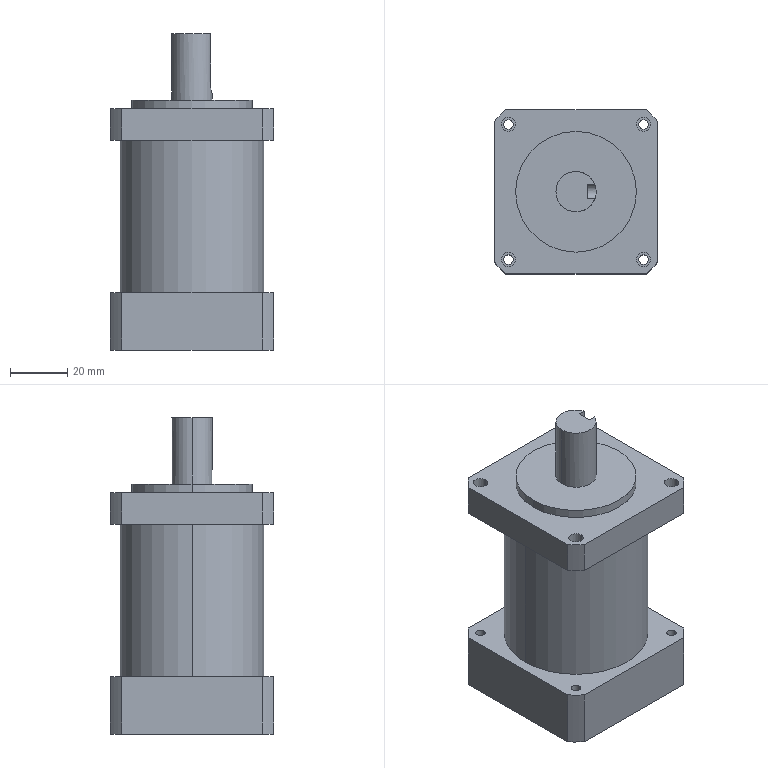Part | STEP file | 57 stepper reducer, 2-stage, ratio 30 | 1 solid | 54 faces | box 57 x 57 x 110 mm | volume 202914 mm3 | cylinder 35 | plane 19 | commonest cylinder face diameters 5 x9 3.3 x8 75 x8 8 x2 14 x2 38 x2